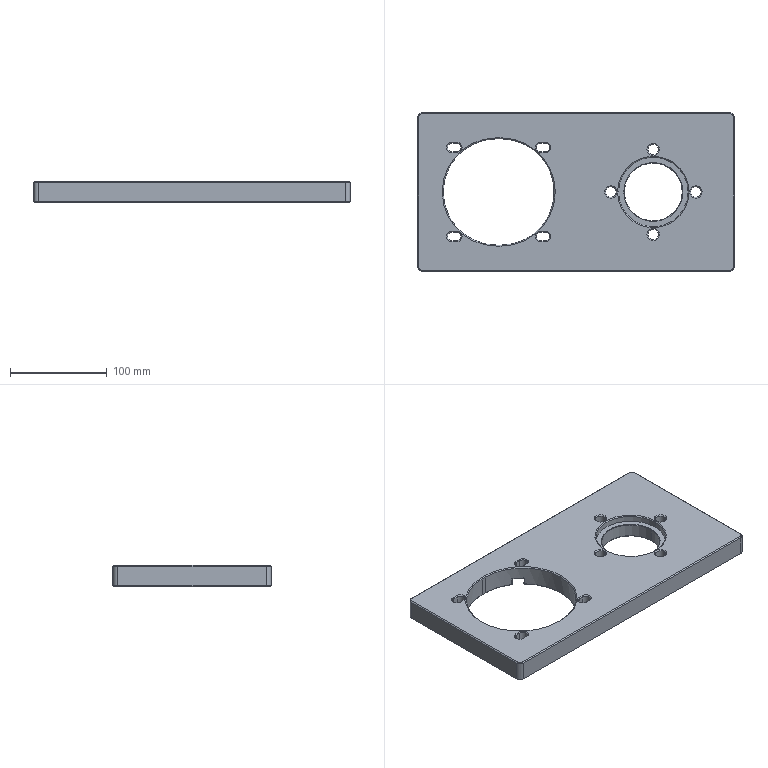NC program | NX | posted with a generic post | part box 328 x 164 x 22 mm
Lines 32 to 855 of 5416:
(HOLE_MILLING , TOOL : D10C)
N56 T10 M6
N58 G54
N60 G17 G0 G90 X-80. Y44. S3500 M3
N62 G43 Z30. H10
N64 Z0.5
N66 G94 G3 X-81.995 Y45.995 R1.995 F1000.
N68 X-83.99 Y44. R1.995
N70 X-83.99 Y44. Z0.3 I3.99 J0. F2500.
N72 X-83.99 Y44. Z0.1 I3.99 J0.
N74 X-83.99 Y44. Z-0.1 I3.99 J0.
N76 X-83.99 Y44. Z-0.3 I3.99 J0.
N78 X-83.99 Y44. Z-0.5 I3.99 J0.
N80 X-83.99 Y44. Z-0.7 I3.99 J0.
N82 X-83.99 Y44. Z-0.9 I3.99 J0.
N84 X-83.99 Y44. Z-1.1 I3.99 J0.
N86 X-83.99 Y44. Z-1.3 I3.99 J0.
N88 X-83.99 Y44. Z-1.5 I3.99 J0.
N90 X-83.99 Y44. Z-1.7 I3.99 J0.
N92 X-83.99 Y44. Z-1.9 I3.99 J0.
N94 X-83.99 Y44. Z-2.1 I3.99 J0.
N96 X-83.99 Y44. Z-2.3 I3.99 J0.
N98 X-83.99 Y44. Z-2.5 I3.99 J0.
N100 X-83.99 Y44. Z-2.7 I3.99 J0.
N102 X-83.99 Y44. Z-2.9 I3.99 J0.
N104 X-83.99 Y44. Z-3.1 I3.99 J0.
N106 X-83.99 Y44. Z-3.3 I3.99 J0.
N108 X-83.99 Y44. Z-3.5 I3.99 J0.
N110 X-83.99 Y44. Z-3.7 I3.99 J0.
N112 X-83.99 Y44. Z-3.9 I3.99 J0.
N114 X-83.99 Y44. Z-4.1 I3.99 J0.
N116 X-83.99 Y44. Z-4.3 I3.99 J0.
N118 X-83.99 Y44. Z-4.5 I3.99 J0.
N120 X-83.99 Y44. Z-4.7 I3.99 J0.
N122 X-83.99 Y44. Z-4.9 I3.99 J0.
N124 X-83.99 Y44. Z-5.1 I3.99 J0.
N126 X-83.99 Y44. Z-5.3 I3.99 J0.
N128 X-83.99 Y44. Z-5.5 I3.99 J0.
N130 X-83.99 Y44. Z-5.7 I3.99 J0.
N132 X-83.99 Y44. Z-5.9 I3.99 J0.
N134 X-83.99 Y44. Z-6.1 I3.99 J0.
N136 X-83.99 Y44. Z-6.3 I3.99 J0.
N138 X-83.99 Y44. Z-6.5 I3.99 J0.
N140 X-83.99 Y44. Z-6.7 I3.99 J0.
N142 X-83.99 Y44. Z-6.9 I3.99 J0.
N144 X-83.99 Y44. Z-7.1 I3.99 J0.
N146 X-83.99 Y44. Z-7.3 I3.99 J0.
N148 X-83.99 Y44. Z-7.5 I3.99 J0.
N150 X-83.99 Y44. Z-7.7 I3.99 J0.
N152 X-83.99 Y44. Z-7.9 I3.99 J0.
N154 X-83.99 Y44. Z-8.1 I3.99 J0.
N156 X-83.99 Y44. Z-8.3 I3.99 J0.
N158 X-83.99 Y44. Z-8.5 I3.99 J0.
N160 X-83.99 Y44. Z-8.7 I3.99 J0.
N162 X-83.99 Y44. Z-8.9 I3.99 J0.
N164 X-83.99 Y44. Z-9.1 I3.99 J0.
N166 X-83.99 Y44. Z-9.3 I3.99 J0.
N168 X-83.99 Y44. Z-9.5 I3.99 J0.
N170 X-83.99 Y44. Z-9.7 I3.99 J0.
N172 X-83.99 Y44. Z-9.9 I3.99 J0.
N174 X-83.99 Y44. Z-10.1 I3.99 J0.
N176 X-83.99 Y44. Z-10.3 I3.99 J0.
N178 X-83.99 Y44. Z-10.5 I3.99 J0.
N180 X-83.99 Y44. Z-10.7 I3.99 J0.
N182 X-83.99 Y44. Z-10.9 I3.99 J0.
N184 X-83.99 Y44. Z-11.1 I3.99 J0.
N186 X-83.99 Y44. Z-11.3 I3.99 J0.
N188 X-83.99 Y44. Z-11.5 I3.99 J0.
N190 X-83.99 Y44. Z-11.7 I3.99 J0.
N192 X-83.99 Y44. Z-11.9 I3.99 J0.
N194 X-76.01 Y44. Z-12. I3.99 J0.
N196 X-80. Y47.99 R3.99
N198 X-76.01 Y44. R-3.99
N200 X-78.005 Y45.995 R1.995
N202 X-80. Y44. R1.995
N204 G0 Z30.
N206 X-36. Y0.
N208 Z0.5
N210 G3 X-37.995 Y1.995 R1.995 F1000.
N212 X-39.99 Y0. R1.995
N214 X-39.99 Y0. Z0.3 I3.99 J0. F2500.
N216 X-39.99 Y0. Z0.1 I3.99 J0.
N218 X-39.99 Y0. Z-0.1 I3.99 J0.
N220 X-39.99 Y0. Z-0.3 I3.99 J0.
N222 X-39.99 Y0. Z-0.5 I3.99 J0.
N224 X-39.99 Y0. Z-0.7 I3.99 J0.
N226 X-39.99 Y0. Z-0.9 I3.99 J0.
N228 X-39.99 Y0. Z-1.1 I3.99 J0.
N230 X-39.99 Y0. Z-1.3 I3.99 J0.
N232 X-39.99 Y0. Z-1.5 I3.99 J0.
N234 X-39.99 Y0. Z-1.7 I3.99 J0.
N236 X-39.99 Y0. Z-1.9 I3.99 J0.
N238 X-39.99 Y0. Z-2.1 I3.99 J0.
N240 X-39.99 Y0. Z-2.3 I3.99 J0.
N242 X-39.99 Y0. Z-2.5 I3.99 J0.
N244 X-39.99 Y0. Z-2.7 I3.99 J0.
N246 X-39.99 Y0. Z-2.9 I3.99 J0.
N248 X-39.99 Y0. Z-3.1 I3.99 J0.
N250 X-39.99 Y0. Z-3.3 I3.99 J0.
N252 X-39.99 Y0. Z-3.5 I3.99 J0.
N254 X-39.99 Y0. Z-3.7 I3.99 J0.
N256 X-39.99 Y0. Z-3.9 I3.99 J0.
N258 X-39.99 Y0. Z-4.1 I3.99 J0.
N260 X-39.99 Y0. Z-4.3 I3.99 J0.
N262 X-39.99 Y0. Z-4.5 I3.99 J0.
N264 X-39.99 Y0. Z-4.7 I3.99 J0.
N266 X-39.99 Y0. Z-4.9 I3.99 J0.
N268 X-39.99 Y0. Z-5.1 I3.99 J0.
N270 X-39.99 Y0. Z-5.3 I3.99 J0.
N272 X-39.99 Y0. Z-5.5 I3.99 J0.
N274 X-39.99 Y0. Z-5.7 I3.99 J0.
N276 X-39.99 Y0. Z-5.9 I3.99 J0.
N278 X-39.99 Y0. Z-6.1 I3.99 J0.
N280 X-39.99 Y0. Z-6.3 I3.99 J0.
N282 X-39.99 Y0. Z-6.5 I3.99 J0.
N284 X-39.99 Y0. Z-6.7 I3.99 J0.
N286 X-39.99 Y0. Z-6.9 I3.99 J0.
N288 X-39.99 Y0. Z-7.1 I3.99 J0.
N290 X-39.99 Y0. Z-7.3 I3.99 J0.
N292 X-39.99 Y0. Z-7.5 I3.99 J0.
N294 X-39.99 Y0. Z-7.7 I3.99 J0.
N296 X-39.99 Y0. Z-7.9 I3.99 J0.
N298 X-39.99 Y0. Z-8.1 I3.99 J0.
N300 X-39.99 Y0. Z-8.3 I3.99 J0.
N302 X-39.99 Y0. Z-8.5 I3.99 J0.
N304 X-39.99 Y0. Z-8.7 I3.99 J0.
N306 X-39.99 Y0. Z-8.9 I3.99 J0.
N308 X-39.99 Y0. Z-9.1 I3.99 J0.
N310 X-39.99 Y0. Z-9.3 I3.99 J0.
N312 X-39.99 Y0. Z-9.5 I3.99 J0.
N314 X-39.99 Y0. Z-9.7 I3.99 J0.
N316 X-39.99 Y0. Z-9.9 I3.99 J0.
N318 X-39.99 Y0. Z-10.1 I3.99 J0.
N320 X-39.99 Y0. Z-10.3 I3.99 J0.
N322 X-39.99 Y0. Z-10.5 I3.99 J0.
N324 X-39.99 Y0. Z-10.7 I3.99 J0.
N326 X-39.99 Y0. Z-10.9 I3.99 J0.
N328 X-39.99 Y0. Z-11.1 I3.99 J0.
N330 X-39.99 Y0. Z-11.3 I3.99 J0.
N332 X-39.99 Y0. Z-11.5 I3.99 J0.
N334 X-39.99 Y0. Z-11.7 I3.99 J0.
N336 X-39.99 Y0. Z-11.9 I3.99 J0.
N338 X-32.01 Y0. Z-12. I3.99 J0.
N340 X-36. Y3.99 R3.99
N342 X-32.01 Y0. R-3.99
N344 X-34.005 Y1.995 R1.995
N346 X-36. Y0. R1.995
N348 G0 Z30.
N350 X-80. Y-44.
N352 Z0.5
N354 G3 X-81.995 Y-42.005 R1.995 F1000.
N356 X-83.99 Y-44. R1.995
N358 X-83.99 Y-44. Z0.3 I3.99 J0. F2500.
N360 X-83.99 Y-44. Z0.1 I3.99 J0.
N362 X-83.99 Y-44. Z-0.1 I3.99 J0.
N364 X-83.99 Y-44. Z-0.3 I3.99 J0.
N366 X-83.99 Y-44. Z-0.5 I3.99 J0.
N368 X-83.99 Y-44. Z-0.7 I3.99 J0.
N370 X-83.99 Y-44. Z-0.9 I3.99 J0.
N372 X-83.99 Y-44. Z-1.1 I3.99 J0.
N374 X-83.99 Y-44. Z-1.3 I3.99 J0.
N376 X-83.99 Y-44. Z-1.5 I3.99 J0.
N378 X-83.99 Y-44. Z-1.7 I3.99 J0.
N380 X-83.99 Y-44. Z-1.9 I3.99 J0.
N382 X-83.99 Y-44. Z-2.1 I3.99 J0.
N384 X-83.99 Y-44. Z-2.3 I3.99 J0.
N386 X-83.99 Y-44. Z-2.5 I3.99 J0.
N388 X-83.99 Y-44. Z-2.7 I3.99 J0.
N390 X-83.99 Y-44. Z-2.9 I3.99 J0.
N392 X-83.99 Y-44. Z-3.1 I3.99 J0.
N394 X-83.99 Y-44. Z-3.3 I3.99 J0.
N396 X-83.99 Y-44. Z-3.5 I3.99 J0.
N398 X-83.99 Y-44. Z-3.7 I3.99 J0.
N400 X-83.99 Y-44. Z-3.9 I3.99 J0.
N402 X-83.99 Y-44. Z-4.1 I3.99 J0.
N404 X-83.99 Y-44. Z-4.3 I3.99 J0.
N406 X-83.99 Y-44. Z-4.5 I3.99 J0.
N408 X-83.99 Y-44. Z-4.7 I3.99 J0.
N410 X-83.99 Y-44. Z-4.9 I3.99 J0.
N412 X-83.99 Y-44. Z-5.1 I3.99 J0.
N414 X-83.99 Y-44. Z-5.3 I3.99 J0.
N416 X-83.99 Y-44. Z-5.5 I3.99 J0.
N418 X-83.99 Y-44. Z-5.7 I3.99 J0.
N420 X-83.99 Y-44. Z-5.9 I3.99 J0.
N422 X-83.99 Y-44. Z-6.1 I3.99 J0.
N424 X-83.99 Y-44. Z-6.3 I3.99 J0.
N426 X-83.99 Y-44. Z-6.5 I3.99 J0.
N428 X-83.99 Y-44. Z-6.7 I3.99 J0.
N430 X-83.99 Y-44. Z-6.9 I3.99 J0.
N432 X-83.99 Y-44. Z-7.1 I3.99 J0.
N434 X-83.99 Y-44. Z-7.3 I3.99 J0.
N436 X-83.99 Y-44. Z-7.5 I3.99 J0.
N438 X-83.99 Y-44. Z-7.7 I3.99 J0.
N440 X-83.99 Y-44. Z-7.9 I3.99 J0.
N442 X-83.99 Y-44. Z-8.1 I3.99 J0.
N444 X-83.99 Y-44. Z-8.3 I3.99 J0.
N446 X-83.99 Y-44. Z-8.5 I3.99 J0.
N448 X-83.99 Y-44. Z-8.7 I3.99 J0.
N450 X-83.99 Y-44. Z-8.9 I3.99 J0.
N452 X-83.99 Y-44. Z-9.1 I3.99 J0.
N454 X-83.99 Y-44. Z-9.3 I3.99 J0.
N456 X-83.99 Y-44. Z-9.5 I3.99 J0.
N458 X-83.99 Y-44. Z-9.7 I3.99 J0.
N460 X-83.99 Y-44. Z-9.9 I3.99 J0.
N462 X-83.99 Y-44. Z-10.1 I3.99 J0.
N464 X-83.99 Y-44. Z-10.3 I3.99 J0.
N466 X-83.99 Y-44. Z-10.5 I3.99 J0.
N468 X-83.99 Y-44. Z-10.7 I3.99 J0.
N470 X-83.99 Y-44. Z-10.9 I3.99 J0.
N472 X-83.99 Y-44. Z-11.1 I3.99 J0.
N474 X-83.99 Y-44. Z-11.3 I3.99 J0.
N476 X-83.99 Y-44. Z-11.5 I3.99 J0.
N478 X-83.99 Y-44. Z-11.7 I3.99 J0.
N480 X-83.99 Y-44. Z-11.9 I3.99 J0.
N482 X-76.01 Y-44. Z-12. I3.99 J0.
N484 X-80. Y-40.01 R3.99
N486 X-76.01 Y-44. R-3.99
N488 X-78.005 Y-42.005 R1.995
N490 X-80. Y-44. R1.995
N492 G0 Z30.
N494 X-124. Y0.
N496 Z0.5
N498 G3 X-125.995 Y1.995 R1.995 F1000.
N500 X-127.99 Y0. R1.995
N502 X-127.99 Y0. Z0.3 I3.99 J0. F2500.
N504 X-127.99 Y0. Z0.1 I3.99 J0.
N506 X-127.99 Y0. Z-0.1 I3.99 J0.
N508 X-127.99 Y0. Z-0.3 I3.99 J0.
N510 X-127.99 Y0. Z-0.5 I3.99 J0.
N512 X-127.99 Y0. Z-0.7 I3.99 J0.
N514 X-127.99 Y0. Z-0.9 I3.99 J0.
N516 X-127.99 Y0. Z-1.1 I3.99 J0.
N518 X-127.99 Y0. Z-1.3 I3.99 J0.
N520 X-127.99 Y0. Z-1.5 I3.99 J0.
N522 X-127.99 Y0. Z-1.7 I3.99 J0.
N524 X-127.99 Y0. Z-1.9 I3.99 J0.
N526 X-127.99 Y0. Z-2.1 I3.99 J0.
N528 X-127.99 Y0. Z-2.3 I3.99 J0.
N530 X-127.99 Y0. Z-2.5 I3.99 J0.
N532 X-127.99 Y0. Z-2.7 I3.99 J0.
N534 X-127.99 Y0. Z-2.9 I3.99 J0.
N536 X-127.99 Y0. Z-3.1 I3.99 J0.
N538 X-127.99 Y0. Z-3.3 I3.99 J0.
N540 X-127.99 Y0. Z-3.5 I3.99 J0.
N542 X-127.99 Y0. Z-3.7 I3.99 J0.
N544 X-127.99 Y0. Z-3.9 I3.99 J0.
N546 X-127.99 Y0. Z-4.1 I3.99 J0.
N548 X-127.99 Y0. Z-4.3 I3.99 J0.
N550 X-127.99 Y0. Z-4.5 I3.99 J0.
N552 X-127.99 Y0. Z-4.7 I3.99 J0.
N554 X-127.99 Y0. Z-4.9 I3.99 J0.
N556 X-127.99 Y0. Z-5.1 I3.99 J0.
N558 X-127.99 Y0. Z-5.3 I3.99 J0.
N560 X-127.99 Y0. Z-5.5 I3.99 J0.
N562 X-127.99 Y0. Z-5.7 I3.99 J0.
N564 X-127.99 Y0. Z-5.9 I3.99 J0.
N566 X-127.99 Y0. Z-6.1 I3.99 J0.
N568 X-127.99 Y0. Z-6.3 I3.99 J0.
N570 X-127.99 Y0. Z-6.5 I3.99 J0.
N572 X-127.99 Y0. Z-6.7 I3.99 J0.
N574 X-127.99 Y0. Z-6.9 I3.99 J0.
N576 X-127.99 Y0. Z-7.1 I3.99 J0.
N578 X-127.99 Y0. Z-7.3 I3.99 J0.
N580 X-127.99 Y0. Z-7.5 I3.99 J0.
N582 X-127.99 Y0. Z-7.7 I3.99 J0.
N584 X-127.99 Y0. Z-7.9 I3.99 J0.
N586 X-127.99 Y0. Z-8.1 I3.99 J0.
N588 X-127.99 Y0. Z-8.3 I3.99 J0.
N590 X-127.99 Y0. Z-8.5 I3.99 J0.
N592 X-127.99 Y0. Z-8.7 I3.99 J0.
N594 X-127.99 Y0. Z-8.9 I3.99 J0.
N596 X-127.99 Y0. Z-9.1 I3.99 J0.
N598 X-127.99 Y0. Z-9.3 I3.99 J0.
N600 X-127.99 Y0. Z-9.5 I3.99 J0.
N602 X-127.99 Y0. Z-9.7 I3.99 J0.
N604 X-127.99 Y0. Z-9.9 I3.99 J0.
N606 X-127.99 Y0. Z-10.1 I3.99 J0.
N608 X-127.99 Y0. Z-10.3 I3.99 J0.
N610 X-127.99 Y0. Z-10.5 I3.99 J0.
N612 X-127.99 Y0. Z-10.7 I3.99 J0.
N614 X-127.99 Y0. Z-10.9 I3.99 J0.
N616 X-127.99 Y0. Z-11.1 I3.99 J0.
N618 X-127.99 Y0. Z-11.3 I3.99 J0.
N620 X-127.99 Y0. Z-11.5 I3.99 J0.
N622 X-127.99 Y0. Z-11.7 I3.99 J0.
N624 X-127.99 Y0. Z-11.9 I3.99 J0.
N626 X-120.01 Y0. Z-12. I3.99 J0.
N628 X-124. Y3.99 R3.99
N630 X-120.01 Y0. R-3.99
N632 X-122.005 Y1.995 R1.995
N634 X-124. Y0. R1.995
N636 G0 Z30.
(ZLEVEL_PROFILE_COPY_1 , TOOL : D10C)
N638 X40.671 Y-32.376 S3000
N640 Z-0.6
N642 G1 X40.541 Y-32.81 F1000.
N644 G3 X40.769 Y-33.783 R1.
N646 G1 X40.979 Y-34.007 F2500.
N648 X41.203 Y-34.246
N650 X41.272 Y-34.323
N652 X41.282 Y-34.331
N654 G2 X41.905 Y-35.176 R9.436
N656 X42.555 Y-36.639 R6.652
N658 X42.803 Y-38.209 R6.745
N660 X42.634 Y-39.791 R6.895
N662 X41.926 Y-41.524 R6.789
N664 X41.179 Y-42.506 R8.918
N666 X40.181 Y-43.367 R6.207
N668 G1 X39.977 Y-43.509
N670 G2 X38.546 Y-44.177 R6.78
N672 X36.863 Y-44.462 R6.701
N674 G1 X28.531
N676 X28.523 Y-44.469
N678 X28.23 Y-44.498
N680 X28.175 Y-44.512
N682 X27.935 Y-44.59
N684 G3 X27.398 Y-44.99 R1.532
N686 G1 X27.176 Y-45.342
N688 X27.055 Y-45.789
N690 X27.069 Y-46.235
N692 X27.118 Y-46.427
N694 X27.193 Y-46.623
N696 G3 X27.597 Y-47.127 R1.377
N698 X28.531 Y-47.455 R1.574
N700 G1 Y-47.462
N702 X39.544
N704 X39.55 Y-47.456
N706 X39.727 Y-47.444
N708 G3 X40.468 Y-47.13 R1.645
N710 G1 X40.811 Y-46.744
N712 X40.846 Y-46.681
N714 X41.006 Y-46.235
N716 X41.052 Y-45.994
N718 G2 X41.319 Y-44.963 R8.476
N720 G1 X41.343 Y-44.896
N722 X41.543 Y-44.418
N724 G2 X41.994 Y-43.619 R11.374
N726 X43.05 Y-42.416 R6.701
N728 X44.758 Y-41.35 R6.864
N730 G1 X44.831 Y-41.335
N732 X45.296 Y-41.179
N734 X45.671 Y-41.072
N736 X45.684 Y-41.066
N738 G2 X47.206 Y-40.91 R6.738
N740 X49.159 Y-41.273 R6.647
N742 G1 X49.88 Y-41.586
N744 X50.233 Y-41.796
N746 G3 X51.233 Y-41.81 R1.
N748 G1 X51.685 Y-41.558
N750 G0 X40.673 Y-32.376 Z-0.8
N752 G1 X40.542 Y-32.809 F1000.
N754 G3 X40.77 Y-33.783 R1.
N756 G1 X40.979 Y-34.006 F2500.
N758 X41.203 Y-34.245
N760 X41.282 Y-34.331
N762 G2 X41.905 Y-35.176 R8.989
N764 X42.555 Y-36.639 R6.607
N766 X42.803 Y-38.217 R6.634
N768 X42.634 Y-39.791 R6.807
N770 X41.919 Y-41.535 R6.685
N772 X41.179 Y-42.506 R8.678
N774 X39.977 Y-43.509 R6.706
N776 X38.546 Y-44.177 R6.698
N778 X36.855 Y-44.462 R6.608
N780 G1 X28.531
N782 X28.523 Y-44.469
N784 G3 X28.173 Y-44.513 R1.583
N786 G1 X27.97 Y-44.579
N788 G3 X27.398 Y-44.99 R1.46
N790 G1 X27.176 Y-45.342
N792 X27.055 Y-45.789
N794 X27.069 Y-46.235
N796 X27.118 Y-46.427
N798 X27.175 Y-46.578
N800 G3 X27.632 Y-47.154 R1.377
N802 X28.531 Y-47.455 R1.574
N804 G1 Y-47.462
N806 X39.544
N808 X39.55 Y-47.456
N810 X39.727 Y-47.444
N812 G3 X40.468 Y-47.13 R1.645
N814 G1 X40.811 Y-46.744
N816 X40.846 Y-46.681
N818 X41.006 Y-46.235
N820 X41.062 Y-45.945
N822 G2 X41.319 Y-44.963 R7.696
N824 G1 X41.343 Y-44.896
N826 X41.543 Y-44.418
N828 G2 X41.994 Y-43.619 R10.723
N830 X43.05 Y-42.416 R6.63
N832 X44.75 Y-41.356 R6.728
N834 X45.684 Y-41.066 R21.266
N836 X47.206 Y-40.91 R6.642
N838 X49.092 Y-41.25 R6.594
N840 G1 X49.289 Y-41.329
N842 G2 X50.141 Y-41.74 R9.632
N844 G1 X50.233 Y-41.796
N846 G3 X51.233 Y-41.816 R1.
N848 G1 X51.692 Y-41.564
N850 G0 X41.255 Y-32.826 Z-1.
N852 G1 X41.08 Y-33.346 F1000.
N854 G3 X41.278 Y-34.326 R1.
N856 G2 X36.703 Y-44.462 R6.1 F2500.
N858 G1 X28.538
N860 G3 X27.038 Y-45.962 R1.5
N862 X28.538 Y-47.462 R1.5
N864 G1 X39.538
N866 G3 X41.024 Y-46.168 R1.5
N868 G2 X50.229 Y-41.793 R6.1
N870 G1 X50.381 Y-41.888
N872 G3 X51.38 Y-41.939 R1.
N874 G1 X51.907 Y-41.669
N876 G0 X41.255 Y-32.825 Z-1.2
N878 G1 X41.08 Y-33.346 F1000.
N880 G3 X41.278 Y-34.326 R1.
N882 G2 X42.803 Y-38.365 R6.1 F2500.
N884 X36.703 Y-44.462 R6.1
N886 G1 X28.538
N888 G3 X27.038 Y-45.962 R1.5
N890 X28.538 Y-47.462 R1.5
N892 G1 X39.538
N894 G3 X41.024 Y-46.168 R1.5
N896 G2 X50.205 Y-41.778 R6.1
N898 G1 X50.381 Y-41.888
N900 G3 X51.38 Y-41.938 R1.
N902 G1 X51.908 Y-41.668
N904 G0 X41.255 Y-32.825 Z-1.4
N906 G1 X41.08 Y-33.346 F1000.
N908 G3 X41.278 Y-34.326 R1.
N910 G2 X42.803 Y-38.365 R6.1 F2500.
N912 X36.703 Y-44.462 R6.1
N914 G1 X28.538
N916 G3 X27.038 Y-45.962 R1.5
N918 X28.538 Y-47.462 R1.5
N920 G1 X39.538
N922 G3 X41.024 Y-46.168 R1.5
N924 G2 X50.205 Y-41.778 R6.1
N926 G1 X50.381 Y-41.888
N928 G3 X51.38 Y-41.938 R1.
N930 G1 X51.908 Y-41.668
N932 G0 X41.255 Y-32.825 Z-1.6
N934 G1 X41.08 Y-33.346 F1000.
N936 G3 X41.278 Y-34.326 R1.
N938 G2 X42.803 Y-38.365 R6.1 F2500.
N940 X36.703 Y-44.462 R6.1
N942 G1 X28.538
N944 G3 X27.038 Y-45.962 R1.5
N946 X28.538 Y-47.462 R1.5
N948 G1 X39.538
N950 G3 X41.024 Y-46.168 R1.5
N952 G2 X50.205 Y-41.778 R6.1
N954 G1 X50.381 Y-41.888
N956 G3 X51.38 Y-41.938 R1.
N958 G1 X51.908 Y-41.668
N960 G0 X41.255 Y-32.825 Z-1.8
N962 G1 X41.08 Y-33.346 F1000.
N964 G3 X41.278 Y-34.326 R1.
N966 G2 X42.803 Y-38.365 R6.1 F2500.
N968 X36.703 Y-44.462 R6.1
N970 G1 X28.538
N972 G3 X27.038 Y-45.962 R1.5
N974 X28.538 Y-47.462 R1.5
N976 G1 X39.538
N978 G3 X41.024 Y-46.168 R1.5
N980 G2 X50.205 Y-41.778 R6.1
N982 G1 X50.381 Y-41.888
N984 G3 X51.38 Y-41.938 R1.
N986 G1 X51.908 Y-41.668
N988 G0 X41.255 Y-32.825 Z-2.
N990 G1 X41.08 Y-33.346 F1000.
N992 G3 X41.278 Y-34.326 R1.
N994 G2 X42.803 Y-38.365 R6.1 F2500.
N996 X36.703 Y-44.462 R6.1
N998 G1 X28.538
N1000 G3 X27.038 Y-45.962 R1.5
N1002 X28.538 Y-47.462 R1.5
N1004 G1 X39.538
N1006 G3 X41.024 Y-46.168 R1.5
N1008 G2 X50.205 Y-41.778 R6.1
N1010 G1 X50.381 Y-41.888
N1012 G3 X51.38 Y-41.938 R1.
N1014 G1 X51.908 Y-41.668
N1016 G0 X41.255 Y-32.825 Z-2.2
N1018 G1 X41.08 Y-33.346 F1000.
N1020 G3 X41.278 Y-34.326 R1.
N1022 G2 X42.803 Y-38.365 R6.1 F2500.
N1024 X36.703 Y-44.462 R6.1
N1026 G1 X28.538
N1028 G3 X27.038 Y-45.962 R1.5
N1030 X28.538 Y-47.462 R1.5
N1032 G1 X39.538
N1034 G3 X41.024 Y-46.168 R1.5
N1036 G2 X50.205 Y-41.778 R6.1
N1038 G1 X50.381 Y-41.888
N1040 G3 X51.38 Y-41.938 R1.
N1042 G1 X51.908 Y-41.668
N1044 G0 X41.255 Y-32.825 Z-2.4
N1046 G1 X41.08 Y-33.346 F1000.
N1048 G3 X41.278 Y-34.326 R1.
N1050 G2 X42.803 Y-38.365 R6.1 F2500.
N1052 X36.703 Y-44.462 R6.1
N1054 G1 X28.538
N1056 G3 X27.038 Y-45.962 R1.5
N1058 X28.538 Y-47.462 R1.5
N1060 G1 X39.538
N1062 G3 X41.024 Y-46.168 R1.5
N1064 G2 X50.205 Y-41.778 R6.1
N1066 G1 X50.381 Y-41.888
N1068 G3 X51.38 Y-41.938 R1.
N1070 G1 X51.908 Y-41.668
N1072 G0 X41.255 Y-32.825 Z-2.6
N1074 G1 X41.08 Y-33.346 F1000.
N1076 G3 X41.278 Y-34.326 R1.
N1078 G2 X42.803 Y-38.365 R6.1 F2500.
N1080 X36.703 Y-44.462 R6.1
N1082 G1 X28.538
N1084 G3 X27.038 Y-45.962 R1.5
N1086 X28.538 Y-47.462 R1.5
N1088 G1 X39.538
N1090 G3 X41.024 Y-46.168 R1.5
N1092 G2 X50.205 Y-41.778 R6.1
N1094 G1 X50.381 Y-41.888
N1096 G3 X51.38 Y-41.938 R1.
N1098 G1 X51.908 Y-41.668
N1100 G0 X41.255 Y-32.825 Z-2.8
N1102 G1 X41.08 Y-33.346 F1000.
N1104 G3 X41.278 Y-34.326 R1.
N1106 G2 X42.803 Y-38.365 R6.1 F2500.
N1108 X36.703 Y-44.462 R6.1
N1110 G1 X28.538
N1112 G3 X27.038 Y-45.962 R1.5
N1114 X28.538 Y-47.462 R1.5
N1116 G1 X39.538
N1118 G3 X41.024 Y-46.168 R1.5
N1120 G2 X50.205 Y-41.778 R6.1
N1122 G1 X50.23 Y-41.792
N1124 X50.381 Y-41.888
N1126 G3 X51.38 Y-41.938 R1.
N1128 G1 X51.908 Y-41.668
N1130 G0 X41.255 Y-32.825 Z-3.
N1132 G1 X41.08 Y-33.346 F1000.
N1134 G3 X41.278 Y-34.326 R1.
N1136 G2 X42.803 Y-38.365 R6.1 F2500.
N1138 X36.703 Y-44.462 R6.1
N1140 G1 X28.538
N1142 G3 X27.038 Y-45.962 R1.5
N1144 X28.538 Y-47.462 R1.5
N1146 G1 X39.538
N1148 G3 X41.024 Y-46.168 R1.5
N1150 G2 X50.205 Y-41.778 R6.1
N1152 G1 X50.23 Y-41.792
N1154 X50.381 Y-41.888
N1156 G3 X51.38 Y-41.938 R1.
N1158 G1 X51.908 Y-41.668
N1160 G0 X41.255 Y-32.825 Z-3.2
N1162 G1 X41.08 Y-33.346 F1000.
N1164 G3 X41.278 Y-34.326 R1.
N1166 G2 X42.803 Y-38.365 R6.1 F2500.
N1168 X36.703 Y-44.462 R6.1
N1170 G1 X28.538
N1172 G3 X27.038 Y-45.962 R1.5
N1174 X28.538 Y-47.462 R1.5
N1176 G1 X39.538
N1178 G3 X41.024 Y-46.168 R1.5
N1180 G2 X50.205 Y-41.778 R6.1
N1182 G1 X50.23 Y-41.792
N1184 X50.381 Y-41.888
N1186 G3 X51.38 Y-41.938 R1.
N1188 G1 X51.908 Y-41.668
N1190 G0 X41.255 Y-32.825 Z-3.4
N1192 G1 X41.08 Y-33.346 F1000.
N1194 G3 X41.278 Y-34.326 R1.
N1196 G2 X42.803 Y-38.365 R6.1 F2500.
N1198 X36.703 Y-44.462 R6.1
N1200 G1 X28.538
N1202 G3 X27.038 Y-45.962 R1.5
N1204 X28.538 Y-47.462 R1.5
N1206 G1 X39.538
N1208 G3 X41.024 Y-46.168 R1.5
N1210 G2 X50.205 Y-41.778 R6.1
N1212 G1 X50.23 Y-41.792
N1214 X50.381 Y-41.888
N1216 G3 X51.38 Y-41.938 R1.
N1218 G1 X51.908 Y-41.668
N1220 G0 X41.255 Y-32.825 Z-3.6
N1222 G1 X41.08 Y-33.346 F1000.
N1224 G3 X41.278 Y-34.326 R1.
N1226 G2 X42.803 Y-38.365 R6.1 F2500.
N1228 X36.703 Y-44.462 R6.1
N1230 G1 X28.538
N1232 G3 X27.038 Y-45.962 R1.5
N1234 X28.538 Y-47.462 R1.5
N1236 G1 X39.538
N1238 G3 X41.024 Y-46.168 R1.5
N1240 G2 X50.205 Y-41.778 R6.1
N1242 G1 X50.23 Y-41.792
N1244 X50.381 Y-41.888
N1246 G3 X51.38 Y-41.938 R1.
N1248 G1 X51.908 Y-41.668
N1250 G0 X41.255 Y-32.825 Z-3.8
N1252 G1 X41.08 Y-33.346 F1000.
N1254 G3 X41.278 Y-34.326 R1.
N1256 G2 X42.803 Y-38.365 R6.1 F2500.
N1258 X36.703 Y-44.462 R6.1
N1260 G1 X28.538
N1262 G3 X27.038 Y-45.962 R1.5
N1264 X28.538 Y-47.462 R1.5
N1266 G1 X39.538
N1268 G3 X41.024 Y-46.168 R1.5
N1270 G2 X50.205 Y-41.778 R6.1
N1272 G1 X50.23 Y-41.792
N1274 X50.381 Y-41.888
N1276 G3 X51.38 Y-41.938 R1.
N1278 G1 X51.908 Y-41.668
N1280 G0 X41.255 Y-32.825 Z-4.
N1282 G1 X41.08 Y-33.346 F1000.
N1284 G3 X41.278 Y-34.326 R1.
N1286 G2 X42.803 Y-38.365 R6.1 F2500.
N1288 X36.703 Y-44.462 R6.1
N1290 G1 X28.538
N1292 G3 X27.038 Y-45.962 R1.5
N1294 X28.538 Y-47.462 R1.5
N1296 G1 X39.538
N1298 G3 X41.024 Y-46.168 R1.5
N1300 G2 X50.205 Y-41.778 R6.1
N1302 G1 X50.23 Y-41.792
N1304 X50.381 Y-41.888
N1306 G3 X51.38 Y-41.938 R1.
N1308 G1 X51.908 Y-41.668
N1310 G0 X41.255 Y-32.825 Z-4.2
N1312 G1 X41.08 Y-33.346 F1000.
N1314 G3 X41.278 Y-34.326 R1.
N1316 G2 X42.803 Y-38.365 R6.1 F2500.
N1318 X36.703 Y-44.462 R6.1
N1320 G1 X28.538
N1322 G3 X27.038 Y-45.962 R1.5
N1324 X28.538 Y-47.462 R1.5
N1326 G1 X39.538
N1328 G3 X41.024 Y-46.168 R1.5
N1330 G2 X50.205 Y-41.778 R6.1
N1332 G1 X50.239 Y-41.797
N1334 X50.381 Y-41.888
N1336 G3 X51.38 Y-41.938 R1.
N1338 G1 X51.908 Y-41.668
N1340 G0 X41.255 Y-32.825 Z-4.4
N1342 G1 X41.08 Y-33.346 F1000.
N1344 G3 X41.278 Y-34.326 R1.
N1346 G2 X42.803 Y-38.365 R6.1 F2500.
N1348 X36.703 Y-44.462 R6.1
N1350 G1 X28.538
N1352 G3 X27.038 Y-45.962 R1.5
N1354 X28.538 Y-47.462 R1.5
N1356 G1 X39.538
N1358 G3 X41.024 Y-46.168 R1.5
N1360 G2 X50.205 Y-41.778 R6.1
N1362 G1 X50.239 Y-41.797
N1364 X50.381 Y-41.888
N1366 G3 X51.38 Y-41.938 R1.
N1368 G1 X51.908 Y-41.668
N1370 G0 X41.255 Y-32.825 Z-4.6
N1372 G1 X41.08 Y-33.346 F1000.
N1374 G3 X41.278 Y-34.326 R1.
N1376 G2 X42.803 Y-38.365 R6.1 F2500.
N1378 X36.703 Y-44.462 R6.1
N1380 G1 X28.538
N1382 G3 X27.038 Y-45.962 R1.5
N1384 X28.538 Y-47.462 R1.5
N1386 G1 X39.538
N1388 G3 X41.024 Y-46.168 R1.5
N1390 G2 X50.205 Y-41.778 R6.1
N1392 G1 X50.239 Y-41.797
N1394 X50.381 Y-41.888
N1396 G3 X51.38 Y-41.938 R1.
N1398 G1 X51.908 Y-41.668
N1400 G0 X41.255 Y-32.825 Z-4.8
N1402 G1 X41.08 Y-33.346 F1000.
N1404 G3 X41.278 Y-34.326 R1.
N1406 G2 X42.803 Y-38.365 R6.1 F2500.
N1408 X36.703 Y-44.462 R6.1
N1410 G1 X28.538
N1412 G3 X27.038 Y-45.962 R1.5
N1414 X28.538 Y-47.462 R1.5
N1416 G1 X39.538
N1418 G3 X41.024 Y-46.168 R1.5
N1420 G2 X50.205 Y-41.778 R6.1
N1422 G1 X50.222 Y-41.786
N1424 X50.381 Y-41.888
N1426 G3 X51.38 Y-41.938 R1.
N1428 G1 X51.908 Y-41.668
N1430 G0 X41.255 Y-32.825 Z-5.
N1432 G1 X41.08 Y-33.346 F1000.
N1434 G3 X41.278 Y-34.326 R1.
N1436 G2 X42.803 Y-38.365 R6.1 F2500.
N1438 X36.703 Y-44.462 R6.1
N1440 G1 X28.538
N1442 G3 X27.038 Y-45.962 R1.5
N1444 X28.538 Y-47.462 R1.5
N1446 G1 X39.538
N1448 G3 X41.024 Y-46.168 R1.5
N1450 G2 X50.205 Y-41.778 R6.1
N1452 G1 X50.222 Y-41.786
N1454 X50.381 Y-41.888
N1456 G3 X51.38 Y-41.938 R1.
N1458 G1 X51.908 Y-41.668
N1460 G0 X41.255 Y-32.825 Z-5.2
N1462 G1 X41.08 Y-33.346 F1000.
N1464 G3 X41.278 Y-34.326 R1.
N1466 G2 X42.803 Y-38.365 R6.1 F2500.
N1468 X36.703 Y-44.462 R6.1
N1470 G1 X28.538
N1472 G3 X27.038 Y-45.962 R1.5
N1474 X28.538 Y-47.462 R1.5
N1476 G1 X39.538
N1478 G3 X41.024 Y-46.168 R1.5
N1480 G2 X50.205 Y-41.778 R6.1
N1482 G1 X50.222 Y-41.786
N1484 X50.381 Y-41.888
N1486 G3 X51.38 Y-41.938 R1.
N1488 G1 X51.908 Y-41.668
N1490 G0 X41.255 Y-32.825 Z-5.4
N1492 G1 X41.08 Y-33.346 F1000.
N1494 G3 X41.278 Y-34.326 R1.
N1496 G2 X42.803 Y-38.365 R6.1 F2500.
N1498 X36.703 Y-44.462 R6.1
N1500 G1 X28.538
N1502 G3 X27.038 Y-45.962 R1.5
N1504 X28.538 Y-47.462 R1.5
N1506 G1 X39.538
N1508 G3 X41.024 Y-46.168 R1.5
N1510 G2 X50.205 Y-41.778 R6.1
N1512 G1 X50.222 Y-41.786
N1514 X50.381 Y-41.888
N1516 G3 X51.38 Y-41.938 R1.
N1518 G1 X51.908 Y-41.668
N1520 G0 X41.255 Y-32.825 Z-5.6
N1522 G1 X41.08 Y-33.346 F1000.
N1524 G3 X41.278 Y-34.326 R1.
N1526 G2 X42.803 Y-38.365 R6.1 F2500.
N1528 X36.703 Y-44.462 R6.1
N1530 G1 X28.538
N1532 G3 X27.038 Y-45.962 R1.5
N1534 X28.538 Y-47.462 R1.5
N1536 G1 X39.538
N1538 G3 X41.024 Y-46.168 R1.5
N1540 G2 X50.205 Y-41.778 R6.1
N1542 G1 X50.222 Y-41.786
N1544 X50.381 Y-41.888
N1546 G3 X51.38 Y-41.938 R1.
N1548 G1 X51.908 Y-41.668
N1550 G0 X41.255 Y-32.825 Z-5.8
N1552 G1 X41.08 Y-33.346 F1000.
N1554 G3 X41.278 Y-34.326 R1.
N1556 G2 X42.803 Y-38.365 R6.1 F2500.
N1558 X36.703 Y-44.462 R6.1
N1560 G1 X28.538
N1562 G3 X27.038 Y-45.962 R1.5
N1564 X28.538 Y-47.462 R1.5
N1566 G1 X39.538
N1568 G3 X41.024 Y-46.168 R1.5
N1570 G2 X50.205 Y-41.778 R6.1
N1572 G1 X50.222 Y-41.786
N1574 X50.381 Y-41.888
N1576 G3 X51.38 Y-41.938 R1.
N1578 G1 X51.908 Y-41.668
N1580 G0 X41.255 Y-32.825 Z-6.
N1582 G1 X41.08 Y-33.346 F1000.
N1584 G3 X41.278 Y-34.326 R1.
N1586 G2 X42.803 Y-38.365 R6.1 F2500.
N1588 X36.703 Y-44.462 R6.1
N1590 G1 X28.538
N1592 G3 X27.038 Y-45.962 R1.5
N1594 X28.538 Y-47.462 R1.5
N1596 G1 X39.538
N1598 G3 X41.024 Y-46.168 R1.5
N1600 G2 X50.205 Y-41.778 R6.1
N1602 G1 X50.222 Y-41.786
N1604 X50.381 Y-41.888
N1606 G3 X51.38 Y-41.938 R1.
N1608 G1 X51.908 Y-41.668
N1610 G0 X41.255 Y-32.825 Z-6.2
N1612 G1 X41.08 Y-33.346 F1000.
N1614 G3 X41.278 Y-34.326 R1.
N1616 G2 X42.803 Y-38.365 R6.1 F2500.
N1618 X36.703 Y-44.462 R6.1
N1620 G1 X28.538
N1622 G3 X27.038 Y-45.962 R1.5
N1624 X28.538 Y-47.462 R1.5
N1626 G1 X39.538
N1628 G3 X41.024 Y-46.168 R1.5
N1630 G2 X50.205 Y-41.778 R6.1
N1632 G1 X50.212 Y-41.782
N1634 X50.222 Y-41.786
N1636 X50.381 Y-41.888
N1638 G3 X51.38 Y-41.938 R1.
N1640 G1 X51.908 Y-41.668
N1642 G0 X41.255 Y-32.825 Z-6.4
N1644 G1 X41.08 Y-33.346 F1000.
N1646 G3 X41.278 Y-34.326 R1.
N1648 G2 X42.803 Y-38.365 R6.1 F2500.
N1650 X36.703 Y-44.462 R6.1
N1652 G1 X28.538
N1654 G3 X27.038 Y-45.962 R1.5
N1656 X28.538 Y-47.462 R1.5
N1658 G1 X39.538
N1660 G3 X41.024 Y-46.168 R1.5
N1662 G2 X50.205 Y-41.778 R6.1
N1664 G1 X50.212 Y-41.782
N1666 X50.222 Y-41.785
N1668 X50.381 Y-41.888
N1670 G3 X51.38 Y-41.938 R1.
N1672 G1 X51.908 Y-41.668
N1674 G0 X41.255 Y-32.825 Z-6.6
N1676 G1 X41.08 Y-33.346 F1000.
N1678 G3 X41.278 Y-34.326 R1.
N1680 G2 X42.803 Y-38.365 R6.1 F2500.
N1682 X36.703 Y-44.462 R6.1
N1684 G1 X28.538
N1686 G3 X27.038 Y-45.962 R1.5
N1688 X28.538 Y-47.462 R1.5
N1690 G1 X39.538